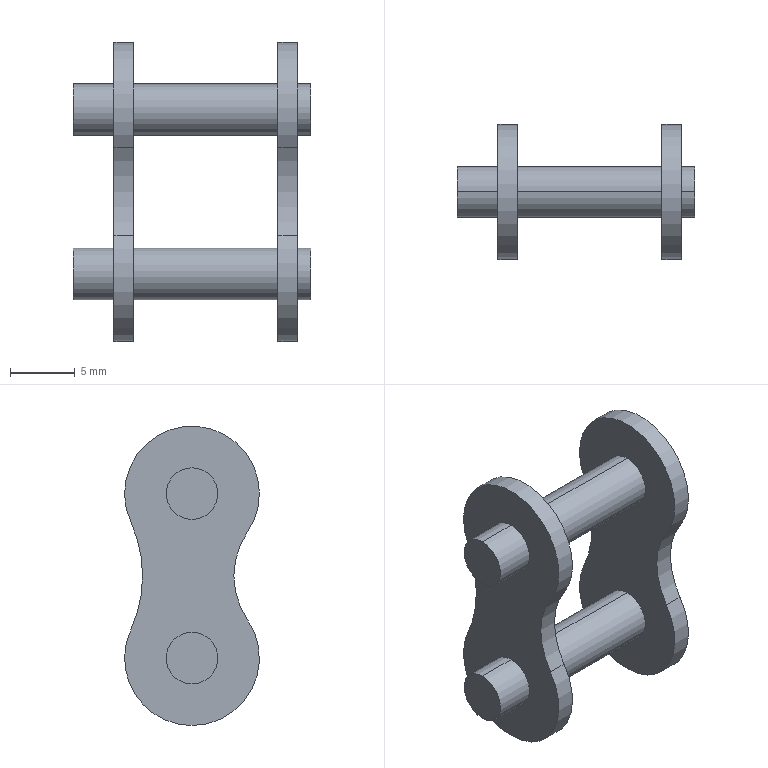Part | STEP file | 1.6 m_VMF01-40-4-A-001 | 1 solid | 30 faces | box 18.36 x 10.41 x 23.11 mm | volume 962.85 mm3 | cylinder 22 | plane 8 | commonest cylinder face diameters 3.98 x12 10.41 x6 12 x2 20 x2
STEP:
#1=CARTESIAN_POINT('',(-10.23,0.,-14.69));
#2=VERTEX_POINT('',#1);
#3=CARTESIAN_POINT('',(-10.23,0.,-10.71));
#4=VERTEX_POINT('',#3);
#5=CARTESIAN_POINT('',(-10.23,0.,-12.7));
#6=DIRECTION('',(1.,0.,0.));
#7=DIRECTION('',(0.,0.,-1.));
#8=AXIS2_PLACEMENT_3D('',#5,#6,#7);
#9=CIRCLE('',#8,1.99);
#10=EDGE_CURVE('',#2,#4,#9,.T.);
#11=ORIENTED_EDGE('',*,*,#10,.T.);
#12=CARTESIAN_POINT('',(-7.075,0.,-10.71));
#13=VERTEX_POINT('',#12);
#14=CARTESIAN_POINT('',(8.13,0.,-10.71));
#15=DIRECTION('',(1.,0.,0.));
#16=VECTOR('',#15,1000.);
#17=LINE('',#14,#16);
#18=EDGE_CURVE('',#4,#13,#17,.T.);
#19=ORIENTED_EDGE('',*,*,#18,.T.);
#20=CARTESIAN_POINT('',(-7.075,0.,-14.69));
#21=VERTEX_POINT('',#20);
#22=CARTESIAN_POINT('',(-7.075,0.,-12.7));
#23=DIRECTION('',(-1.,0.,0.));
#24=DIRECTION('',(0.,0.,-1.));
#25=AXIS2_PLACEMENT_3D('',#22,#23,#24);
#26=CIRCLE('',#25,1.99);
#27=EDGE_CURVE('',#13,#21,#26,.T.);
#28=ORIENTED_EDGE('',*,*,#27,.T.);
#29=CARTESIAN_POINT('',(8.13,0.,-14.69));
#30=DIRECTION('',(1.,0.,0.));
#31=VECTOR('',#30,1000.);
#32=LINE('',#29,#31);
#33=EDGE_CURVE('',#2,#21,#32,.T.);
#34=ORIENTED_EDGE('',*,*,#33,.F.);
#35=EDGE_LOOP('',(#11,#19,#28,#34));
#36=FACE_OUTER_BOUND('',#35,.T.);
#37=CARTESIAN_POINT('',(8.13,0.,-12.7));
#38=DIRECTION('',(1.,0.,0.));
#39=DIRECTION('',(0.,0.,-1.));
#40=AXIS2_PLACEMENT_3D('',#37,#38,#39);
#41=CYLINDRICAL_SURFACE('',#40,1.99);
#42=ADVANCED_FACE('',(#36),#41,.T.);
#43=CARTESIAN_POINT('',(-7.075,-4.288,-9.75));
#44=VERTEX_POINT('',#43);
#45=CARTESIAN_POINT('',(-7.075,0.,-17.905));
#46=VERTEX_POINT('',#45);
#47=CARTESIAN_POINT('',(-7.075,0.,-12.7));
#48=DIRECTION('',(1.,0.,0.));
#49=DIRECTION('',(0.,0.,-1.));
#50=AXIS2_PLACEMENT_3D('',#47,#48,#49);
#51=CIRCLE('',#50,5.205);
#52=EDGE_CURVE('',#44,#46,#51,.T.);
#53=ORIENTED_EDGE('',*,*,#52,.T.);
#54=CARTESIAN_POINT('',(-5.585,0.,-17.905));
#55=VERTEX_POINT('',#54);
#56=CARTESIAN_POINT('',(7.075,0.,-17.905));
#57=DIRECTION('',(1.,0.,0.));
#58=VECTOR('',#57,1000.);
#59=LINE('',#56,#58);
#60=EDGE_CURVE('',#46,#55,#59,.T.);
#61=ORIENTED_EDGE('',*,*,#60,.T.);
#62=CARTESIAN_POINT('',(-5.585,-4.288,-9.75));
#63=VERTEX_POINT('',#62);
#64=CARTESIAN_POINT('',(-5.585,0.,-12.7));
#65=DIRECTION('',(-1.,0.,0.));
#66=DIRECTION('',(0.,0.,-1.));
#67=AXIS2_PLACEMENT_3D('',#64,#65,#66);
#68=CIRCLE('',#67,5.205);
#69=EDGE_CURVE('',#55,#63,#68,.T.);
#70=ORIENTED_EDGE('',*,*,#69,.T.);
#71=CARTESIAN_POINT('',(7.075,-4.288,-9.75));
#72=DIRECTION('',(-1.,0.,0.));
#73=VECTOR('',#72,1000.);
#74=LINE('',#71,#73);
#75=EDGE_CURVE('',#63,#44,#74,.T.);
#76=ORIENTED_EDGE('',*,*,#75,.T.);
#77=EDGE_LOOP('',(#53,#61,#70,#76));
#78=FACE_OUTER_BOUND('',#77,.T.);
#79=CARTESIAN_POINT('',(7.075,0.,-12.7));
#80=DIRECTION('',(1.,0.,0.));
#81=DIRECTION('',(0.,0.,-1.));
#82=AXIS2_PLACEMENT_3D('',#79,#80,#81);
#83=CYLINDRICAL_SURFACE('',#82,5.205);
#84=ADVANCED_FACE('',(#78),#83,.T.);
#85=CARTESIAN_POINT('',(-10.23,0.,-1.99));
#86=VERTEX_POINT('',#85);
#87=CARTESIAN_POINT('',(-10.23,0.,1.99));
#88=VERTEX_POINT('',#87);
#89=CARTESIAN_POINT('',(-10.23,0.,0.));
#90=DIRECTION('',(1.,0.,0.));
#91=DIRECTION('',(0.,0.,-1.));
#92=AXIS2_PLACEMENT_3D('',#89,#90,#91);
#93=CIRCLE('',#92,1.99);
#94=EDGE_CURVE('',#86,#88,#93,.T.);
#95=ORIENTED_EDGE('',*,*,#94,.T.);
#96=CARTESIAN_POINT('',(-7.075,0.,1.99));
#97=VERTEX_POINT('',#96);
#98=CARTESIAN_POINT('',(8.13,0.,1.99));
#99=DIRECTION('',(1.,0.,0.));
#100=VECTOR('',#99,1000.);
#101=LINE('',#98,#100);
#102=EDGE_CURVE('',#88,#97,#101,.T.);
#103=ORIENTED_EDGE('',*,*,#102,.T.);
#104=CARTESIAN_POINT('',(-7.075,0.,-1.99));
#105=VERTEX_POINT('',#104);
#106=CARTESIAN_POINT('',(-7.075,0.,0.));
#107=DIRECTION('',(-1.,0.,0.));
#108=DIRECTION('',(0.,0.,-1.));
#109=AXIS2_PLACEMENT_3D('',#106,#107,#108);
#110=CIRCLE('',#109,1.99);
#111=EDGE_CURVE('',#97,#105,#110,.T.);
#112=ORIENTED_EDGE('',*,*,#111,.T.);
#113=CARTESIAN_POINT('',(8.13,0.,-1.99));
#114=DIRECTION('',(1.,0.,0.));
#115=VECTOR('',#114,1000.);
#116=LINE('',#113,#115);
#117=EDGE_CURVE('',#86,#105,#116,.T.);
#118=ORIENTED_EDGE('',*,*,#117,.F.);
#119=EDGE_LOOP('',(#95,#103,#112,#118));
#120=FACE_OUTER_BOUND('',#119,.T.);
#121=CARTESIAN_POINT('',(8.13,0.,0.));
#122=DIRECTION('',(1.,0.,0.));
#123=DIRECTION('',(0.,0.,-1.));
#124=AXIS2_PLACEMENT_3D('',#121,#122,#123);
#125=CYLINDRICAL_SURFACE('',#124,1.99);
#126=ADVANCED_FACE('',(#120),#125,.T.);
#127=CARTESIAN_POINT('',(-5.585,0.,1.99));
#128=VERTEX_POINT('',#127);
#129=CARTESIAN_POINT('',(-5.585,0.,-1.99));
#130=VERTEX_POINT('',#129);
#131=CARTESIAN_POINT('',(-5.585,0.,0.));
#132=DIRECTION('',(-1.,0.,0.));
#133=DIRECTION('',(0.,0.,-1.));
#134=AXIS2_PLACEMENT_3D('',#131,#132,#133);
#135=CIRCLE('',#134,1.99);
#136=EDGE_CURVE('',#128,#130,#135,.T.);
#137=ORIENTED_EDGE('',*,*,#136,.F.);
#138=CARTESIAN_POINT('',(5.585,0.,1.99));
#139=VERTEX_POINT('',#138);
#140=CARTESIAN_POINT('',(5.585,0.,1.99));
#141=DIRECTION('',(1.,0.,0.));
#142=VECTOR('',#141,1000.);
#143=LINE('',#140,#142);
#144=EDGE_CURVE('',#128,#139,#143,.T.);
#145=ORIENTED_EDGE('',*,*,#144,.T.);
#146=CARTESIAN_POINT('',(5.585,0.,-1.99));
#147=VERTEX_POINT('',#146);
#148=CARTESIAN_POINT('',(5.585,0.,0.));
#149=DIRECTION('',(-1.,0.,0.));
#150=DIRECTION('',(0.,0.,-1.));
#151=AXIS2_PLACEMENT_3D('',#148,#149,#150);
#152=CIRCLE('',#151,1.99);
#153=EDGE_CURVE('',#139,#147,#152,.T.);
#154=ORIENTED_EDGE('',*,*,#153,.T.);
#155=CARTESIAN_POINT('',(5.585,0.,-1.99));
#156=DIRECTION('',(1.,0.,0.));
#157=VECTOR('',#156,1000.);
#158=LINE('',#155,#157);
#159=EDGE_CURVE('',#130,#147,#158,.T.);
#160=ORIENTED_EDGE('',*,*,#159,.F.);
#161=EDGE_LOOP('',(#137,#145,#154,#160));
#162=FACE_OUTER_BOUND('',#161,.T.);
#163=CARTESIAN_POINT('',(5.585,0.,0.));
#164=DIRECTION('',(1.,0.,0.));
#165=DIRECTION('',(0.,0.,-1.));
#166=AXIS2_PLACEMENT_3D('',#163,#164,#165);
#167=CYLINDRICAL_SURFACE('',#166,1.99);
#168=ADVANCED_FACE('',(#162),#167,.T.);
#169=CARTESIAN_POINT('',(-5.585,0.,-10.71));
#170=VERTEX_POINT('',#169);
#171=CARTESIAN_POINT('',(-5.585,0.,-14.69));
#172=VERTEX_POINT('',#171);
#173=CARTESIAN_POINT('',(-5.585,0.,-12.7));
#174=DIRECTION('',(-1.,0.,0.));
#175=DIRECTION('',(0.,0.,-1.));
#176=AXIS2_PLACEMENT_3D('',#173,#174,#175);
#177=CIRCLE('',#176,1.99);
#178=EDGE_CURVE('',#170,#172,#177,.T.);
#179=ORIENTED_EDGE('',*,*,#178,.F.);
#180=CARTESIAN_POINT('',(5.585,0.,-10.71));
#181=VERTEX_POINT('',#180);
#182=CARTESIAN_POINT('',(5.585,0.,-10.71));
#183=DIRECTION('',(1.,0.,0.));
#184=VECTOR('',#183,1000.);
#185=LINE('',#182,#184);
#186=EDGE_CURVE('',#170,#181,#185,.T.);
#187=ORIENTED_EDGE('',*,*,#186,.T.);
#188=CARTESIAN_POINT('',(5.585,0.,-14.69));
#189=VERTEX_POINT('',#188);
#190=CARTESIAN_POINT('',(5.585,0.,-12.7));
#191=DIRECTION('',(-1.,0.,0.));
#192=DIRECTION('',(0.,0.,-1.));
#193=AXIS2_PLACEMENT_3D('',#190,#191,#192);
#194=CIRCLE('',#193,1.99);
#195=EDGE_CURVE('',#181,#189,#194,.T.);
#196=ORIENTED_EDGE('',*,*,#195,.T.);
#197=CARTESIAN_POINT('',(5.585,0.,-14.69));
#198=DIRECTION('',(1.,0.,0.));
#199=VECTOR('',#198,1000.);
#200=LINE('',#197,#199);
#201=EDGE_CURVE('',#172,#189,#200,.T.);
#202=ORIENTED_EDGE('',*,*,#201,.F.);
#203=EDGE_LOOP('',(#179,#187,#196,#202));
#204=FACE_OUTER_BOUND('',#203,.T.);
#205=CARTESIAN_POINT('',(5.585,0.,-12.7));
#206=DIRECTION('',(1.,0.,0.));
#207=DIRECTION('',(0.,0.,-1.));
#208=AXIS2_PLACEMENT_3D('',#205,#206,#207);
#209=CYLINDRICAL_SURFACE('',#208,1.99);
#210=ADVANCED_FACE('',(#204),#209,.T.);
#211=CARTESIAN_POINT('',(5.585,-4.288,-9.75));
#212=VERTEX_POINT('',#211);
#213=CARTESIAN_POINT('',(5.585,0.,-17.905));
#214=VERTEX_POINT('',#213);
#215=CARTESIAN_POINT('',(5.585,0.,-12.7));
#216=DIRECTION('',(1.,0.,0.));
#217=DIRECTION('',(0.,0.,-1.));
#218=AXIS2_PLACEMENT_3D('',#215,#216,#217);
#219=CIRCLE('',#218,5.205);
#220=EDGE_CURVE('',#212,#214,#219,.T.);
#221=ORIENTED_EDGE('',*,*,#220,.T.);
#222=CARTESIAN_POINT('',(7.075,0.,-17.905));
#223=VERTEX_POINT('',#222);
#224=CARTESIAN_POINT('',(7.075,0.,-17.905));
#225=DIRECTION('',(1.,0.,0.));
#226=VECTOR('',#225,1000.);
#227=LINE('',#224,#226);
#228=EDGE_CURVE('',#214,#223,#227,.T.);
#229=ORIENTED_EDGE('',*,*,#228,.T.);
#230=CARTESIAN_POINT('',(7.075,-4.288,-9.75));
#231=VERTEX_POINT('',#230);
#232=CARTESIAN_POINT('',(7.075,0.,-12.7));
#233=DIRECTION('',(-1.,0.,0.));
#234=DIRECTION('',(0.,0.,-1.));
#235=AXIS2_PLACEMENT_3D('',#232,#233,#234);
#236=CIRCLE('',#235,5.205);
#237=EDGE_CURVE('',#223,#231,#236,.T.);
#238=ORIENTED_EDGE('',*,*,#237,.T.);
#239=CARTESIAN_POINT('',(7.075,-4.288,-9.75));
#240=DIRECTION('',(-1.,0.,0.));
#241=VECTOR('',#240,1000.);
#242=LINE('',#239,#241);
#243=EDGE_CURVE('',#231,#212,#242,.T.);
#244=ORIENTED_EDGE('',*,*,#243,.T.);
#245=EDGE_LOOP('',(#221,#229,#238,#244));
#246=FACE_OUTER_BOUND('',#245,.T.);
#247=CARTESIAN_POINT('',(7.075,0.,-12.7));
#248=DIRECTION('',(1.,0.,0.));
#249=DIRECTION('',(0.,0.,-1.));
#250=AXIS2_PLACEMENT_3D('',#247,#248,#249);
#251=CYLINDRICAL_SURFACE('',#250,5.205);
#252=ADVANCED_FACE('',(#246),#251,.T.);
#253=CARTESIAN_POINT('',(7.075,0.,-10.71));
#254=VERTEX_POINT('',#253);
#255=CARTESIAN_POINT('',(7.075,0.,-14.69));
#256=VERTEX_POINT('',#255);
#257=CARTESIAN_POINT('',(7.075,0.,-12.7));
#258=DIRECTION('',(-1.,0.,0.));
#259=DIRECTION('',(0.,0.,-1.));
#260=AXIS2_PLACEMENT_3D('',#257,#258,#259);
#261=CIRCLE('',#260,1.99);
#262=EDGE_CURVE('',#254,#256,#261,.T.);
#263=ORIENTED_EDGE('',*,*,#262,.F.);
#264=CARTESIAN_POINT('',(8.13,0.,-10.71));
#265=VERTEX_POINT('',#264);
#266=CARTESIAN_POINT('',(8.13,0.,-10.71));
#267=DIRECTION('',(1.,0.,0.));
#268=VECTOR('',#267,1000.);
#269=LINE('',#266,#268);
#270=EDGE_CURVE('',#254,#265,#269,.T.);
#271=ORIENTED_EDGE('',*,*,#270,.T.);
#272=CARTESIAN_POINT('',(8.13,0.,-14.69));
#273=VERTEX_POINT('',#272);
#274=CARTESIAN_POINT('',(8.13,0.,-12.7));
#275=DIRECTION('',(-1.,0.,0.));
#276=DIRECTION('',(0.,0.,-1.));
#277=AXIS2_PLACEMENT_3D('',#274,#275,#276);
#278=CIRCLE('',#277,1.99);
#279=EDGE_CURVE('',#265,#273,#278,.T.);
#280=ORIENTED_EDGE('',*,*,#279,.T.);
#281=CARTESIAN_POINT('',(8.13,0.,-14.69));
#282=DIRECTION('',(1.,0.,0.));
#283=VECTOR('',#282,1000.);
#284=LINE('',#281,#283);
#285=EDGE_CURVE('',#256,#273,#284,.T.);
#286=ORIENTED_EDGE('',*,*,#285,.F.);
#287=EDGE_LOOP('',(#263,#271,#280,#286));
#288=FACE_OUTER_BOUND('',#287,.T.);
#289=CARTESIAN_POINT('',(8.13,0.,-12.7));
#290=DIRECTION('',(1.,0.,0.));
#291=DIRECTION('',(0.,0.,-1.));
#292=AXIS2_PLACEMENT_3D('',#289,#290,#291);
#293=CYLINDRICAL_SURFACE('',#292,1.99);
#294=ADVANCED_FACE('',(#288),#293,.T.);
#295=CARTESIAN_POINT('',(7.075,0.,1.99));
#296=VERTEX_POINT('',#295);
#297=CARTESIAN_POINT('',(7.075,0.,-1.99));
#298=VERTEX_POINT('',#297);
#299=CARTESIAN_POINT('',(7.075,0.,0.));
#300=DIRECTION('',(-1.,0.,0.));
#301=DIRECTION('',(0.,0.,-1.));
#302=AXIS2_PLACEMENT_3D('',#299,#300,#301);
#303=CIRCLE('',#302,1.99);
#304=EDGE_CURVE('',#296,#298,#303,.T.);
#305=ORIENTED_EDGE('',*,*,#304,.F.);
#306=CARTESIAN_POINT('',(8.13,0.,1.99));
#307=VERTEX_POINT('',#306);
#308=CARTESIAN_POINT('',(8.13,0.,1.99));
#309=DIRECTION('',(1.,0.,0.));
#310=VECTOR('',#309,1000.);
#311=LINE('',#308,#310);
#312=EDGE_CURVE('',#296,#307,#311,.T.);
#313=ORIENTED_EDGE('',*,*,#312,.T.);
#314=CARTESIAN_POINT('',(8.13,0.,-1.99));
#315=VERTEX_POINT('',#314);
#316=CARTESIAN_POINT('',(8.13,0.,0.));
#317=DIRECTION('',(-1.,0.,0.));
#318=DIRECTION('',(0.,0.,-1.));
#319=AXIS2_PLACEMENT_3D('',#316,#317,#318);
#320=CIRCLE('',#319,1.99);
#321=EDGE_CURVE('',#307,#315,#320,.T.);
#322=ORIENTED_EDGE('',*,*,#321,.T.);
#323=CARTESIAN_POINT('',(8.13,0.,-1.99));
#324=DIRECTION('',(1.,0.,0.));
#325=VECTOR('',#324,1000.);
#326=LINE('',#323,#325);
#327=EDGE_CURVE('',#298,#315,#326,.T.);
#328=ORIENTED_EDGE('',*,*,#327,.F.);
#329=EDGE_LOOP('',(#305,#313,#322,#328));
#330=FACE_OUTER_BOUND('',#329,.T.);
#331=CARTESIAN_POINT('',(8.13,0.,0.));
#332=DIRECTION('',(1.,0.,0.));
#333=DIRECTION('',(0.,0.,-1.));
#334=AXIS2_PLACEMENT_3D('',#331,#332,#333);
#335=CYLINDRICAL_SURFACE('',#334,1.99);
#336=ADVANCED_FACE('',(#330),#335,.T.);
#337=CARTESIAN_POINT('',(-7.075,0.,-12.7));
#338=DIRECTION('',(-1.,0.,0.));
#339=DIRECTION('',(0.,0.,-1.));
#340=AXIS2_PLACEMENT_3D('',#337,#338,#339);
#341=CIRCLE('',#340,1.99);
#342=EDGE_CURVE('',#21,#13,#341,.T.);
#343=ORIENTED_EDGE('',*,*,#342,.F.);
#344=ORIENTED_EDGE('',*,*,#27,.F.);
#345=EDGE_LOOP('',(#343,#344));
#346=FACE_BOUND('',#345,.T.);
#347=ORIENTED_EDGE('',*,*,#52,.F.);
#348=CARTESIAN_POINT('',(-7.075,-4.288,-2.95));
#349=VERTEX_POINT('',#348);
#350=CARTESIAN_POINT('',(-7.075,-9.232,-6.35));
#351=DIRECTION('',(-1.,0.,0.));
#352=DIRECTION('',(0.,0.,-1.));
#353=AXIS2_PLACEMENT_3D('',#350,#351,#352);
#354=CIRCLE('',#353,6.);
#355=EDGE_CURVE('',#349,#44,#354,.T.);
#356=ORIENTED_EDGE('',*,*,#355,.F.);
#357=CARTESIAN_POINT('',(-7.075,4.729,-2.174));
#358=VERTEX_POINT('',#357);
#359=CARTESIAN_POINT('',(-7.075,0.,0.));
#360=DIRECTION('',(1.,0.,0.));
#361=DIRECTION('',(0.,0.,-1.));
#362=AXIS2_PLACEMENT_3D('',#359,#360,#361);
#363=CIRCLE('',#362,5.205);
#364=EDGE_CURVE('',#358,#349,#363,.T.);
#365=ORIENTED_EDGE('',*,*,#364,.F.);
#366=CARTESIAN_POINT('',(-7.075,4.729,-10.526));
#367=VERTEX_POINT('',#366);
#368=CARTESIAN_POINT('',(-7.075,13.816,-6.35));
#369=DIRECTION('',(-1.,0.,0.));
#370=DIRECTION('',(0.,0.,-1.));
#371=AXIS2_PLACEMENT_3D('',#368,#369,#370);
#372=CIRCLE('',#371,10.);
#373=EDGE_CURVE('',#367,#358,#372,.T.);
#374=ORIENTED_EDGE('',*,*,#373,.F.);
#375=CARTESIAN_POINT('',(-7.075,0.,-12.7));
#376=DIRECTION('',(1.,0.,0.));
#377=DIRECTION('',(0.,0.,-1.));
#378=AXIS2_PLACEMENT_3D('',#375,#376,#377);
#379=CIRCLE('',#378,5.205);
#380=EDGE_CURVE('',#46,#367,#379,.T.);
#381=ORIENTED_EDGE('',*,*,#380,.F.);
#382=EDGE_LOOP('',(#347,#356,#365,#374,#381));
#383=FACE_OUTER_BOUND('',#382,.T.);
#384=CARTESIAN_POINT('',(-7.075,0.,0.));
#385=DIRECTION('',(-1.,0.,0.));
#386=DIRECTION('',(0.,0.,-1.));
#387=AXIS2_PLACEMENT_3D('',#384,#385,#386);
#388=CIRCLE('',#387,1.99);
#389=EDGE_CURVE('',#105,#97,#388,.T.);
#390=ORIENTED_EDGE('',*,*,#389,.F.);
#391=ORIENTED_EDGE('',*,*,#111,.F.);
#392=EDGE_LOOP('',(#390,#391));
#393=FACE_BOUND('',#392,.T.);
#394=CARTESIAN_POINT('',(-7.075,6.908,-9.525));
#395=DIRECTION('',(1.,0.,0.));
#396=DIRECTION('',(0.,0.,-1.));
#397=AXIS2_PLACEMENT_3D('',#394,#395,#396);
#398=PLANE('',#397);
#399=ADVANCED_FACE('',(#346,#383,#393),#398,.F.);
#400=ORIENTED_EDGE('',*,*,#18,.F.);
#401=CARTESIAN_POINT('',(-10.23,0.,-12.7));
#402=DIRECTION('',(1.,0.,0.));
#403=DIRECTION('',(0.,0.,-1.));
#404=AXIS2_PLACEMENT_3D('',#401,#402,#403);
#405=CIRCLE('',#404,1.99);
#406=EDGE_CURVE('',#4,#2,#405,.T.);
#407=ORIENTED_EDGE('',*,*,#406,.T.);
#408=ORIENTED_EDGE('',*,*,#33,.T.);
#409=ORIENTED_EDGE('',*,*,#342,.T.);
#410=EDGE_LOOP('',(#400,#407,#408,#409));
#411=FACE_OUTER_BOUND('',#410,.T.);
#412=CARTESIAN_POINT('',(8.13,0.,-12.7));
#413=DIRECTION('',(1.,0.,0.));
#414=DIRECTION('',(0.,0.,-1.));
#415=AXIS2_PLACEMENT_3D('',#412,#413,#414);
#416=CYLINDRICAL_SURFACE('',#415,1.99);
#417=ADVANCED_FACE('',(#411),#416,.T.);
#418=CARTESIAN_POINT('',(-5.585,4.729,-10.526));
#419=VERTEX_POINT('',#418);
#420=CARTESIAN_POINT('',(-5.585,4.729,-2.174));
#421=VERTEX_POINT('',#420);
#422=CARTESIAN_POINT('',(-5.585,13.816,-6.35));
#423=DIRECTION('',(-1.,0.,0.));
#424=DIRECTION('',(0.,0.,-1.));
#425=AXIS2_PLACEMENT_3D('',#422,#423,#424);
#426=CIRCLE('',#425,10.);
#427=EDGE_CURVE('',#419,#421,#426,.T.);
#428=ORIENTED_EDGE('',*,*,#427,.F.);
#429=CARTESIAN_POINT('',(7.075,4.729,-10.526));
#430=DIRECTION('',(1.,0.,0.));
#431=VECTOR('',#430,1000.);
#432=LINE('',#429,#431);
#433=EDGE_CURVE('',#367,#419,#432,.T.);
#434=ORIENTED_EDGE('',*,*,#433,.F.);
#435=ORIENTED_EDGE('',*,*,#373,.T.);
#436=CARTESIAN_POINT('',(7.075,4.729,-2.174));
#437=DIRECTION('',(-1.,0.,0.));
#438=VECTOR('',#437,1000.);
#439=LINE('',#436,#438);
#440=EDGE_CURVE('',#421,#358,#439,.T.);
#441=ORIENTED_EDGE('',*,*,#440,.F.);
#442=EDGE_LOOP('',(#428,#434,#435,#441));
#443=FACE_OUTER_BOUND('',#442,.T.);
#444=CARTESIAN_POINT('',(7.075,13.816,-6.35));
#445=DIRECTION('',(1.,0.,0.));
#446=DIRECTION('',(0.,0.,-1.));
#447=AXIS2_PLACEMENT_3D('',#444,#445,#446);
#448=CYLINDRICAL_SURFACE('',#447,10.);
#449=ADVANCED_FACE('',(#443),#448,.F.);
#450=ORIENTED_EDGE('',*,*,#60,.F.);
#451=ORIENTED_EDGE('',*,*,#380,.T.);
#452=ORIENTED_EDGE('',*,*,#433,.T.);
#453=CARTESIAN_POINT('',(-5.585,0.,-12.7));
#454=DIRECTION('',(-1.,0.,0.));
#455=DIRECTION('',(0.,0.,-1.));
#456=AXIS2_PLACEMENT_3D('',#453,#454,#455);
#457=CIRCLE('',#456,5.205);
#458=EDGE_CURVE('',#419,#55,#457,.T.);
#459=ORIENTED_EDGE('',*,*,#458,.T.);
#460=EDGE_LOOP('',(#450,#451,#452,#459));
#461=FACE_OUTER_BOUND('',#460,.T.);
#462=CARTESIAN_POINT('',(7.075,0.,-12.7));
#463=DIRECTION('',(1.,0.,0.));
#464=DIRECTION('',(0.,0.,-1.));
#465=AXIS2_PLACEMENT_3D('',#462,#463,#464);
#466=CYLINDRICAL_SURFACE('',#465,5.205);
#467=ADVANCED_FACE('',(#461),#466,.T.);
#468=CARTESIAN_POINT('',(-5.585,-4.288,-2.95));
#469=VERTEX_POINT('',#468);
#470=CARTESIAN_POINT('',(-5.585,-9.232,-6.35));
#471=DIRECTION('',(-1.,0.,0.));
#472=DIRECTION('',(0.,0.,-1.));
#473=AXIS2_PLACEMENT_3D('',#470,#471,#472);
#474=CIRCLE('',#473,6.);
#475=EDGE_CURVE('',#469,#63,#474,.T.);
#476=ORIENTED_EDGE('',*,*,#475,.F.);
#477=CARTESIAN_POINT('',(7.075,-4.288,-2.95));
#478=DIRECTION('',(1.,0.,0.));
#479=VECTOR('',#478,1000.);
#480=LINE('',#477,#479);
#481=EDGE_CURVE('',#349,#469,#480,.T.);
#482=ORIENTED_EDGE('',*,*,#481,.F.);
#483=ORIENTED_EDGE('',*,*,#355,.T.);
#484=ORIENTED_EDGE('',*,*,#75,.F.);
#485=EDGE_LOOP('',(#476,#482,#483,#484));
#486=FACE_OUTER_BOUND('',#485,.T.);
#487=CARTESIAN_POINT('',(7.075,-9.232,-6.35));
#488=DIRECTION('',(1.,0.,0.));
#489=DIRECTION('',(0.,0.,-1.));
#490=AXIS2_PLACEMENT_3D('',#487,#488,#489);
#491=CYLINDRICAL_SURFACE('',#490,6.);
#492=ADVANCED_FACE('',(#486),#491,.F.);
#493=ORIENTED_EDGE('',*,*,#364,.T.);
#494=ORIENTED_EDGE('',*,*,#481,.T.);
#495=CARTESIAN_POINT('',(-5.585,0.,0.));
#496=DIRECTION('',(-1.,0.,0.));
#497=DIRECTION('',(0.,0.,-1.));
#498=AXIS2_PLACEMENT_3D('',#495,#496,#497);
#499=CIRCLE('',#498,5.205);
#500=EDGE_CURVE('',#469,#421,#499,.T.);
#501=ORIENTED_EDGE('',*,*,#500,.T.);
#502=ORIENTED_EDGE('',*,*,#440,.T.);
#503=EDGE_LOOP('',(#493,#494,#501,#502));
#504=FACE_OUTER_BOUND('',#503,.T.);
#505=CARTESIAN_POINT('',(7.075,0.,0.));
#506=DIRECTION('',(1.,0.,0.));
#507=DIRECTION('',(0.,0.,-1.));
#508=AXIS2_PLACEMENT_3D('',#505,#506,#507);
#509=CYLINDRICAL_SURFACE('',#508,5.205);
#510=ADVANCED_FACE('',(#504),#509,.T.);
#511=ORIENTED_EDGE('',*,*,#102,.F.);
#512=CARTESIAN_POINT('',(-10.23,0.,0.));
#513=DIRECTION('',(1.,0.,0.));
#514=DIRECTION('',(0.,0.,-1.));
#515=AXIS2_PLACEMENT_3D('',#512,#513,#514);
#516=CIRCLE('',#515,1.99);
#517=EDGE_CURVE('',#88,#86,#516,.T.);
#518=ORIENTED_EDGE('',*,*,#517,.T.);
#519=ORIENTED_EDGE('',*,*,#117,.T.);
#520=ORIENTED_EDGE('',*,*,#389,.T.);
#521=EDGE_LOOP('',(#511,#518,#519,#520));
#522=FACE_OUTER_BOUND('',#521,.T.);
#523=CARTESIAN_POINT('',(8.13,0.,0.));
#524=DIRECTION('',(1.,0.,0.));
#525=DIRECTION('',(0.,0.,-1.));
#526=AXIS2_PLACEMENT_3D('',#523,#524,#525);
#527=CYLINDRICAL_SURFACE('',#526,1.99);
#528=ADVANCED_FACE('',(#522),#527,.T.);
#529=ORIENTED_EDGE('',*,*,#10,.F.);
#530=ORIENTED_EDGE('',*,*,#406,.F.);
#531=EDGE_LOOP('',(#529,#530));
#532=FACE_OUTER_BOUND('',#531,.T.);
#533=CARTESIAN_POINT('',(-10.23,0.,-12.7));
#534=DIRECTION('',(1.,0.,0.));
#535=DIRECTION('',(0.,0.,-1.));
#536=AXIS2_PLACEMENT_3D('',#533,#534,#535);
#537=PLANE('',#536);
#538=ADVANCED_FACE('',(#532),#537,.F.);
#539=CARTESIAN_POINT('',(-5.585,0.,0.));
#540=DIRECTION('',(-1.,0.,0.));
#541=DIRECTION('',(0.,0.,-1.));
#542=AXIS2_PLACEMENT_3D('',#539,#540,#541);
#543=CIRCLE('',#542,1.99);
#544=EDGE_CURVE('',#130,#128,#543,.T.);
#545=ORIENTED_EDGE('',*,*,#544,.T.);
#546=ORIENTED_EDGE('',*,*,#136,.T.);
#547=EDGE_LOOP('',(#545,#546));
#548=FACE_BOUND('',#547,.T.);
#549=ORIENTED_EDGE('',*,*,#475,.T.);
#550=ORIENTED_EDGE('',*,*,#69,.F.);
#551=ORIENTED_EDGE('',*,*,#458,.F.);
#552=ORIENTED_EDGE('',*,*,#427,.T.);
#553=ORIENTED_EDGE('',*,*,#500,.F.);
#554=EDGE_LOOP('',(#549,#550,#551,#552,#553));
#555=FACE_OUTER_BOUND('',#554,.T.);
#556=CARTESIAN_POINT('',(-5.585,0.,-12.7));
#557=DIRECTION('',(-1.,0.,0.));
#558=DIRECTION('',(0.,0.,-1.));
#559=AXIS2_PLACEMENT_3D('',#556,#557,#558);
#560=CIRCLE('',#559,1.99);
#561=EDGE_CURVE('',#172,#170,#560,.T.);
#562=ORIENTED_EDGE('',*,*,#561,.T.);
#563=ORIENTED_EDGE('',*,*,#178,.T.);
#564=EDGE_LOOP('',(#562,#563));
#565=FACE_BOUND('',#564,.T.);
#566=CARTESIAN_POINT('',(-5.585,6.908,-9.525));
#567=DIRECTION('',(1.,0.,0.));
#568=DIRECTION('',(0.,0.,-1.));
#569=AXIS2_PLACEMENT_3D('',#566,#567,#568);
#570=PLANE('',#569);
#571=ADVANCED_FACE('',(#548,#555,#565),#570,.T.);
#572=ORIENTED_EDGE('',*,*,#94,.F.);
#573=ORIENTED_EDGE('',*,*,#517,.F.);
#574=EDGE_LOOP('',(#572,#573));
#575=FACE_OUTER_BOUND('',#574,.T.);
#576=CARTESIAN_POINT('',(-10.23,0.,0.));
#577=DIRECTION('',(1.,0.,0.));
#578=DIRECTION('',(0.,0.,-1.));
#579=AXIS2_PLACEMENT_3D('',#576,#577,#578);
#580=PLANE('',#579);
#581=ADVANCED_FACE('',(#575),#580,.F.);
#582=ORIENTED_EDGE('',*,*,#144,.F.);
#583=ORIENTED_EDGE('',*,*,#544,.F.);
#584=ORIENTED_EDGE('',*,*,#159,.T.);
#585=CARTESIAN_POINT('',(5.585,0.,0.));
#586=DIRECTION('',(-1.,0.,0.));
#587=DIRECTION('',(0.,0.,-1.));
#588=AXIS2_PLACEMENT_3D('',#585,#586,#587);
#589=CIRCLE('',#588,1.99);
#590=EDGE_CURVE('',#147,#139,#589,.T.);
#591=ORIENTED_EDGE('',*,*,#590,.T.);
#592=EDGE_LOOP('',(#582,#583,#584,#591));
#593=FACE_OUTER_BOUND('',#592,.T.);
#594=CARTESIAN_POINT('',(5.585,0.,0.));
#595=DIRECTION('',(1.,0.,0.));
#596=DIRECTION('',(0.,0.,-1.));
#597=AXIS2_PLACEMENT_3D('',#594,#595,#596);
#598=CYLINDRICAL_SURFACE('',#597,1.99);
#599=ADVANCED_FACE('',(#593),#598,.T.);
#600=ORIENTED_EDGE('',*,*,#186,.F.);
#601=ORIENTED_EDGE('',*,*,#561,.F.);
#602=ORIENTED_EDGE('',*,*,#201,.T.);
#603=CARTESIAN_POINT('',(5.585,0.,-12.7));
#604=DIRECTION('',(-1.,0.,0.));
#605=DIRECTION('',(0.,0.,-1.));
#606=AXIS2_PLACEMENT_3D('',#603,#604,#605);
#607=CIRCLE('',#606,1.99);
#608=EDGE_CURVE('',#189,#181,#607,.T.);
#609=ORIENTED_EDGE('',*,*,#608,.T.);
#610=EDGE_LOOP('',(#600,#601,#602,#609));
#611=FACE_OUTER_BOUND('',#610,.T.);
#612=CARTESIAN_POINT('',(5.585,0.,-12.7));
#613=DIRECTION('',(1.,0.,0.));
#614=DIRECTION('',(0.,0.,-1.));
#615=AXIS2_PLACEMENT_3D('',#612,#613,#614);
#616=CYLINDRICAL_SURFACE('',#615,1.99);
#617=ADVANCED_FACE('',(#611),#616,.T.);
#618=ORIENTED_EDGE('',*,*,#590,.F.);
#619=ORIENTED_EDGE('',*,*,#153,.F.);
#620=EDGE_LOOP('',(#618,#619));
#621=FACE_BOUND('',#620,.T.);
#622=ORIENTED_EDGE('',*,*,#220,.F.);
#623=CARTESIAN_POINT('',(5.585,-4.288,-2.95));
#624=VERTEX_POINT('',#623);
#625=CARTESIAN_POINT('',(5.585,-9.232,-6.35));
#626=DIRECTION('',(-1.,0.,0.));
#627=DIRECTION('',(0.,0.,-1.));
#628=AXIS2_PLACEMENT_3D('',#625,#626,#627);
#629=CIRCLE('',#628,6.);
#630=EDGE_CURVE('',#624,#212,#629,.T.);
#631=ORIENTED_EDGE('',*,*,#630,.F.);
#632=CARTESIAN_POINT('',(5.585,4.729,-2.174));
#633=VERTEX_POINT('',#632);
#634=CARTESIAN_POINT('',(5.585,0.,0.));
#635=DIRECTION('',(1.,0.,0.));
#636=DIRECTION('',(0.,0.,-1.));
#637=AXIS2_PLACEMENT_3D('',#634,#635,#636);
#638=CIRCLE('',#637,5.205);
#639=EDGE_CURVE('',#633,#624,#638,.T.);
#640=ORIENTED_EDGE('',*,*,#639,.F.);
#641=CARTESIAN_POINT('',(5.585,4.729,-10.526));
#642=VERTEX_POINT('',#641);
#643=CARTESIAN_POINT('',(5.585,13.816,-6.35));
#644=DIRECTION('',(-1.,0.,0.));
#645=DIRECTION('',(0.,0.,-1.));
#646=AXIS2_PLACEMENT_3D('',#643,#644,#645);
#647=CIRCLE('',#646,10.);
#648=EDGE_CURVE('',#642,#633,#647,.T.);
#649=ORIENTED_EDGE('',*,*,#648,.F.);
#650=CARTESIAN_POINT('',(5.585,0.,-12.7));
#651=DIRECTION('',(1.,0.,0.));
#652=DIRECTION('',(0.,0.,-1.));
#653=AXIS2_PLACEMENT_3D('',#650,#651,#652);
#654=CIRCLE('',#653,5.205);
#655=EDGE_CURVE('',#214,#642,#654,.T.);
#656=ORIENTED_EDGE('',*,*,#655,.F.);
#657=EDGE_LOOP('',(#622,#631,#640,#649,#656));
#658=FACE_OUTER_BOUND('',#657,.T.);
#659=ORIENTED_EDGE('',*,*,#608,.F.);
#660=ORIENTED_EDGE('',*,*,#195,.F.);
#661=EDGE_LOOP('',(#659,#660));
#662=FACE_BOUND('',#661,.T.);
#663=CARTESIAN_POINT('',(5.585,6.908,-9.525));
#664=DIRECTION('',(1.,0.,0.));
#665=DIRECTION('',(0.,0.,-1.));
#666=AXIS2_PLACEMENT_3D('',#663,#664,#665);
#667=PLANE('',#666);
#668=ADVANCED_FACE('',(#621,#658,#662),#667,.F.);
#669=CARTESIAN_POINT('',(7.075,4.729,-2.174));
#670=VERTEX_POINT('',#669);
#671=CARTESIAN_POINT('',(7.075,4.729,-2.174));
#672=DIRECTION('',(-1.,0.,0.));
#673=VECTOR('',#672,1000.);
#674=LINE('',#671,#673);
#675=EDGE_CURVE('',#670,#633,#674,.T.);
#676=ORIENTED_EDGE('',*,*,#675,.F.);
#677=CARTESIAN_POINT('',(7.075,4.729,-10.526));
#678=VERTEX_POINT('',#677);
#679=CARTESIAN_POINT('',(7.075,13.816,-6.35));
#680=DIRECTION('',(-1.,0.,0.));
#681=DIRECTION('',(0.,0.,-1.));
#682=AXIS2_PLACEMENT_3D('',#679,#680,#681);
#683=CIRCLE('',#682,10.);
#684=EDGE_CURVE('',#678,#670,#683,.T.);
#685=ORIENTED_EDGE('',*,*,#684,.F.);
#686=CARTESIAN_POINT('',(7.075,4.729,-10.526));
#687=DIRECTION('',(1.,0.,0.));
#688=VECTOR('',#687,1000.);
#689=LINE('',#686,#688);
#690=EDGE_CURVE('',#642,#678,#689,.T.);
#691=ORIENTED_EDGE('',*,*,#690,.F.);
#692=ORIENTED_EDGE('',*,*,#648,.T.);
#693=EDGE_LOOP('',(#676,#685,#691,#692));
#694=FACE_OUTER_BOUND('',#693,.T.);
#695=CARTESIAN_POINT('',(7.075,13.816,-6.35));
#696=DIRECTION('',(1.,0.,0.));
#697=DIRECTION('',(0.,0.,-1.));
#698=AXIS2_PLACEMENT_3D('',#695,#696,#697);
#699=CYLINDRICAL_SURFACE('',#698,10.);
#700=ADVANCED_FACE('',(#694),#699,.F.);
#701=ORIENTED_EDGE('',*,*,#228,.F.);
#702=ORIENTED_EDGE('',*,*,#655,.T.);
#703=ORIENTED_EDGE('',*,*,#690,.T.);
#704=CARTESIAN_POINT('',(7.075,0.,-12.7));
#705=DIRECTION('',(-1.,0.,0.));
#706=DIRECTION('',(0.,0.,-1.));
#707=AXIS2_PLACEMENT_3D('',#704,#705,#706);
#708=CIRCLE('',#707,5.205);
#709=EDGE_CURVE('',#678,#223,#708,.T.);
#710=ORIENTED_EDGE('',*,*,#709,.T.);
#711=EDGE_LOOP('',(#701,#702,#703,#710));
#712=FACE_OUTER_BOUND('',#711,.T.);
#713=CARTESIAN_POINT('',(7.075,0.,-12.7));
#714=DIRECTION('',(1.,0.,0.));
#715=DIRECTION('',(0.,0.,-1.));
#716=AXIS2_PLACEMENT_3D('',#713,#714,#715);
#717=CYLINDRICAL_SURFACE('',#716,5.205);
#718=ADVANCED_FACE('',(#712),#717,.T.);
#719=ORIENTED_EDGE('',*,*,#243,.F.);
#720=CARTESIAN_POINT('',(7.075,-4.288,-2.95));
#721=VERTEX_POINT('',#720);
#722=CARTESIAN_POINT('',(7.075,-9.232,-6.35));
#723=DIRECTION('',(-1.,0.,0.));
#724=DIRECTION('',(0.,0.,-1.));
#725=AXIS2_PLACEMENT_3D('',#722,#723,#724);
#726=CIRCLE('',#725,6.);
#727=EDGE_CURVE('',#721,#231,#726,.T.);
#728=ORIENTED_EDGE('',*,*,#727,.F.);
#729=CARTESIAN_POINT('',(7.075,-4.288,-2.95));
#730=DIRECTION('',(1.,0.,0.));
#731=VECTOR('',#730,1000.);
#732=LINE('',#729,#731);
#733=EDGE_CURVE('',#624,#721,#732,.T.);
#734=ORIENTED_EDGE('',*,*,#733,.F.);
#735=ORIENTED_EDGE('',*,*,#630,.T.);
#736=EDGE_LOOP('',(#719,#728,#734,#735));
#737=FACE_OUTER_BOUND('',#736,.T.);
#738=CARTESIAN_POINT('',(7.075,-9.232,-6.35));
#739=DIRECTION('',(1.,0.,0.));
#740=DIRECTION('',(0.,0.,-1.));
#741=AXIS2_PLACEMENT_3D('',#738,#739,#740);
#742=CYLINDRICAL_SURFACE('',#741,6.);
#743=ADVANCED_FACE('',(#737),#742,.F.);
#744=ORIENTED_EDGE('',*,*,#733,.T.);
#745=CARTESIAN_POINT('',(7.075,0.,0.));
#746=DIRECTION('',(-1.,0.,0.));
#747=DIRECTION('',(0.,0.,-1.));
#748=AXIS2_PLACEMENT_3D('',#745,#746,#747);
#749=CIRCLE('',#748,5.205);
#750=EDGE_CURVE('',#721,#670,#749,.T.);
#751=ORIENTED_EDGE('',*,*,#750,.T.);
#752=ORIENTED_EDGE('',*,*,#675,.T.);
#753=ORIENTED_EDGE('',*,*,#639,.T.);
#754=EDGE_LOOP('',(#744,#751,#752,#753));
#755=FACE_OUTER_BOUND('',#754,.T.);
#756=CARTESIAN_POINT('',(7.075,0.,0.));
#757=DIRECTION('',(1.,0.,0.));
#758=DIRECTION('',(0.,0.,-1.));
#759=AXIS2_PLACEMENT_3D('',#756,#757,#758);
#760=CYLINDRICAL_SURFACE('',#759,5.205);
#761=ADVANCED_FACE('',(#755),#760,.T.);
#762=CARTESIAN_POINT('',(7.075,0.,-12.7));
#763=DIRECTION('',(-1.,0.,0.));
#764=DIRECTION('',(0.,0.,-1.));
#765=AXIS2_PLACEMENT_3D('',#762,#763,#764);
#766=CIRCLE('',#765,1.99);
#767=EDGE_CURVE('',#256,#254,#766,.T.);
#768=ORIENTED_EDGE('',*,*,#767,.T.);
#769=ORIENTED_EDGE('',*,*,#262,.T.);
#770=EDGE_LOOP('',(#768,#769));
#771=FACE_BOUND('',#770,.T.);
#772=ORIENTED_EDGE('',*,*,#727,.T.);
#773=ORIENTED_EDGE('',*,*,#237,.F.);
#774=ORIENTED_EDGE('',*,*,#709,.F.);
#775=ORIENTED_EDGE('',*,*,#684,.T.);
#776=ORIENTED_EDGE('',*,*,#750,.F.);
#777=EDGE_LOOP('',(#772,#773,#774,#775,#776));
#778=FACE_OUTER_BOUND('',#777,.T.);
#779=CARTESIAN_POINT('',(7.075,0.,0.));
#780=DIRECTION('',(-1.,0.,0.));
#781=DIRECTION('',(0.,0.,-1.));
#782=AXIS2_PLACEMENT_3D('',#779,#780,#781);
#783=CIRCLE('',#782,1.99);
#784=EDGE_CURVE('',#298,#296,#783,.T.);
#785=ORIENTED_EDGE('',*,*,#784,.T.);
#786=ORIENTED_EDGE('',*,*,#304,.T.);
#787=EDGE_LOOP('',(#785,#786));
#788=FACE_BOUND('',#787,.T.);
#789=CARTESIAN_POINT('',(7.075,6.908,-9.525));
#790=DIRECTION('',(1.,0.,0.));
#791=DIRECTION('',(0.,0.,-1.));
#792=AXIS2_PLACEMENT_3D('',#789,#790,#791);
#793=PLANE('',#792);
#794=ADVANCED_FACE('',(#771,#778,#788),#793,.T.);
#795=ORIENTED_EDGE('',*,*,#270,.F.);
#796=ORIENTED_EDGE('',*,*,#767,.F.);
#797=ORIENTED_EDGE('',*,*,#285,.T.);
#798=CARTESIAN_POINT('',(8.13,0.,-12.7));
#799=DIRECTION('',(-1.,0.,0.));
#800=DIRECTION('',(0.,0.,-1.));
#801=AXIS2_PLACEMENT_3D('',#798,#799,#800);
#802=CIRCLE('',#801,1.99);
#803=EDGE_CURVE('',#273,#265,#802,.T.);
#804=ORIENTED_EDGE('',*,*,#803,.T.);
#805=EDGE_LOOP('',(#795,#796,#797,#804));
#806=FACE_OUTER_BOUND('',#805,.T.);
#807=CARTESIAN_POINT('',(8.13,0.,-12.7));
#808=DIRECTION('',(1.,0.,0.));
#809=DIRECTION('',(0.,0.,-1.));
#810=AXIS2_PLACEMENT_3D('',#807,#808,#809);
#811=CYLINDRICAL_SURFACE('',#810,1.99);
#812=ADVANCED_FACE('',(#806),#811,.T.);
#813=ORIENTED_EDGE('',*,*,#312,.F.);
#814=ORIENTED_EDGE('',*,*,#784,.F.);
#815=ORIENTED_EDGE('',*,*,#327,.T.);
#816=CARTESIAN_POINT('',(8.13,0.,0.));
#817=DIRECTION('',(-1.,0.,0.));
#818=DIRECTION('',(0.,0.,-1.));
#819=AXIS2_PLACEMENT_3D('',#816,#817,#818);
#820=CIRCLE('',#819,1.99);
#821=EDGE_CURVE('',#315,#307,#820,.T.);
#822=ORIENTED_EDGE('',*,*,#821,.T.);
#823=EDGE_LOOP('',(#813,#814,#815,#822));
#824=FACE_OUTER_BOUND('',#823,.T.);
#825=CARTESIAN_POINT('',(8.13,0.,0.));
#826=DIRECTION('',(1.,0.,0.));
#827=DIRECTION('',(0.,0.,-1.));
#828=AXIS2_PLACEMENT_3D('',#825,#826,#827);
#829=CYLINDRICAL_SURFACE('',#828,1.99);
#830=ADVANCED_FACE('',(#824),#829,.T.);
#831=ORIENTED_EDGE('',*,*,#803,.F.);
#832=ORIENTED_EDGE('',*,*,#279,.F.);
#833=EDGE_LOOP('',(#831,#832));
#834=FACE_OUTER_BOUND('',#833,.T.);
#835=CARTESIAN_POINT('',(8.13,0.,-12.7));
#836=DIRECTION('',(1.,0.,0.));
#837=DIRECTION('',(0.,0.,-1.));
#838=AXIS2_PLACEMENT_3D('',#835,#836,#837);
#839=PLANE('',#838);
#840=ADVANCED_FACE('',(#834),#839,.T.);
#841=ORIENTED_EDGE('',*,*,#821,.F.);
#842=ORIENTED_EDGE('',*,*,#321,.F.);
#843=EDGE_LOOP('',(#841,#842));
#844=FACE_OUTER_BOUND('',#843,.T.);
#845=CARTESIAN_POINT('',(8.13,0.,0.));
#846=DIRECTION('',(1.,0.,0.));
#847=DIRECTION('',(0.,0.,-1.));
#848=AXIS2_PLACEMENT_3D('',#845,#846,#847);
#849=PLANE('',#848);
#850=ADVANCED_FACE('',(#844),#849,.T.);
#851=CLOSED_SHELL('',(#42,#84,#126,#168,#210,#252,#294,#336,#399,#417,#449,#467,#492,#510,#528,#538,#571,#581,#599,#617,#668,#700,#718,#743,#761,#794,#812,#830,#840,#850));
#852=MANIFOLD_SOLID_BREP('',#851);
#853=CARTESIAN_POINT('',(0.,0.,0.));
#854=DIRECTION('',(0.,0.,1.));
#855=DIRECTION('',(1.,0.,0.));
#856=AXIS2_PLACEMENT_3D('',#853,#854,#855);
#857=(LENGTH_UNIT()NAMED_UNIT(*)SI_UNIT(.MILLI.,.METRE.));
#858=UNCERTAINTY_MEASURE_WITH_UNIT(LENGTH_MEASURE(0.00001),#857,'','');
#859=(NAMED_UNIT(*)PLANE_ANGLE_UNIT()SI_UNIT($,.RADIAN.));
#860=(NAMED_UNIT(*)SI_UNIT($,.STERADIAN.)SOLID_ANGLE_UNIT());
#861=(GEOMETRIC_REPRESENTATION_CONTEXT(3)GLOBAL_UNCERTAINTY_ASSIGNED_CONTEXT((#858))GLOBAL_UNIT_ASSIGNED_CONTEXT((#857,#859,#860))REPRESENTATION_CONTEXT('',''));
#862=ADVANCED_BREP_SHAPE_REPRESENTATION('',(#852,#856),#861);